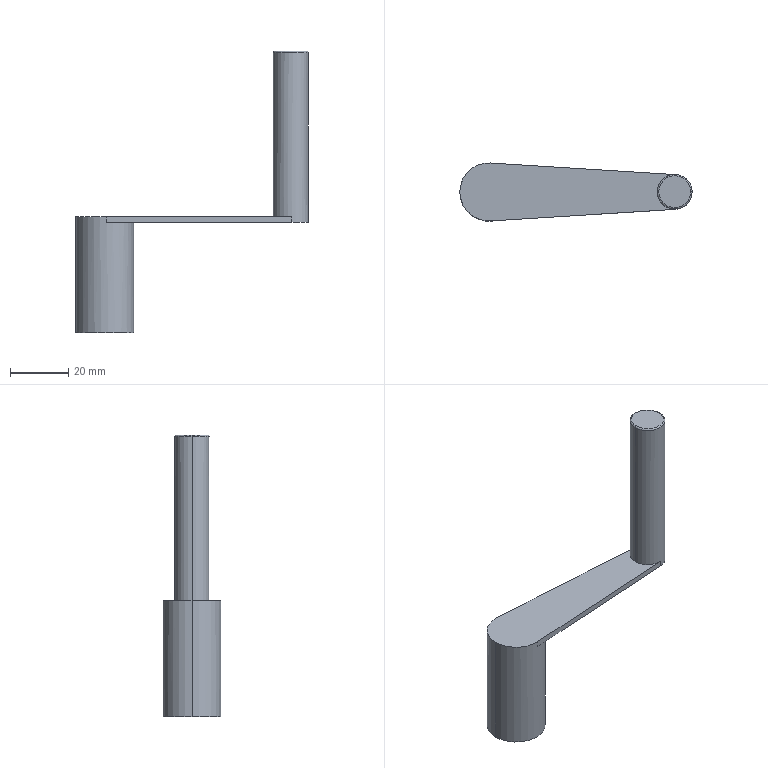Part | STEP file | Z-type Silver Iron Handle | 1 solid | 21 faces | box 80 x 20 x 97 mm | volume 17986 mm3 | plane 11 | cylinder 8 | torus 2 | commonest cylinder face diameters 1 x4 12 x2 20 x2
STEP:
#1=CARTESIAN_POINT('',(0.,0.,0.));
#2=DIRECTION('',(0.,0.,1.));
#3=DIRECTION('',(1.,0.,0.));
#4=AXIS2_PLACEMENT_3D('',#1,#2,#3);
#5=CARTESIAN_POINT('',(58.,0.,96.5));
#6=VERTEX_POINT('',#5);
#7=CARTESIAN_POINT('',(70.,0.,96.5));
#8=VERTEX_POINT('',#7);
#9=CARTESIAN_POINT('',(64.,0.,96.5));
#10=DIRECTION('',(0.,0.,-1.));
#11=DIRECTION('',(1.,0.,0.));
#12=AXIS2_PLACEMENT_3D('',#9,#10,#11);
#13=CIRCLE('',#12,6.);
#14=CARTESIAN_POINT('',(64.,0.,96.5));
#15=DIRECTION('',(0.,0.,1.));
#16=DIRECTION('',(1.,0.,0.));
#17=AXIS2_PLACEMENT_3D('',#14,#15,#16);
#18=TOROIDAL_SURFACE('',#17,5.5,0.5);
#19=CARTESIAN_POINT('',(6.283,0.));
#20=DIRECTION('',(-1.,0.));
#21=VECTOR('',#20,1.);
#22=LINE('',#19,#21);
#23=(GEOMETRIC_REPRESENTATION_CONTEXT(2)PARAMETRIC_REPRESENTATION_CONTEXT()REPRESENTATION_CONTEXT('',''));
#24=DEFINITIONAL_REPRESENTATION('',(#22),#23);
#25=PCURVE('',#18,#24);
#26=CARTESIAN_POINT('',(64.,0.,40.));
#27=DIRECTION('',(0.,0.,-1.));
#28=DIRECTION('',(-1.,0.,0.));
#29=AXIS2_PLACEMENT_3D('',#26,#27,#28);
#30=CYLINDRICAL_SURFACE('',#29,6.);
#31=CARTESIAN_POINT('',(-3.142,-56.5));
#32=DIRECTION('',(1.,0.));
#33=VECTOR('',#32,1.);
#34=LINE('',#31,#33);
#35=(GEOMETRIC_REPRESENTATION_CONTEXT(2)PARAMETRIC_REPRESENTATION_CONTEXT()REPRESENTATION_CONTEXT('',''));
#36=DEFINITIONAL_REPRESENTATION('',(#34),#35);
#37=PCURVE('',#30,#36);
#38=SURFACE_CURVE('',#13,(#25,#37),.PCURVE_S1.);
#39=EDGE_CURVE('',#6,#8,#38,.T.);
#40=ORIENTED_EDGE('',*,*,#39,.F.);
#41=CARTESIAN_POINT('',(58.5,0.,97.));
#42=VERTEX_POINT('',#41);
#43=CARTESIAN_POINT('',(58.5,0.,96.5));
#44=DIRECTION('',(0.,1.,0.));
#45=DIRECTION('',(-1.,0.,0.));
#46=AXIS2_PLACEMENT_3D('',#43,#44,#45);
#47=CIRCLE('',#46,0.5);
#48=CARTESIAN_POINT('',(3.142,0.));
#49=DIRECTION('',(0.,1.));
#50=VECTOR('',#49,1.);
#51=LINE('',#48,#50);
#52=(GEOMETRIC_REPRESENTATION_CONTEXT(2)PARAMETRIC_REPRESENTATION_CONTEXT()REPRESENTATION_CONTEXT('',''));
#53=DEFINITIONAL_REPRESENTATION('',(#51),#52);
#54=PCURVE('',#18,#53);
#55=CARTESIAN_POINT('',(64.,0.,96.5));
#56=DIRECTION('',(0.,0.,1.));
#57=DIRECTION('',(1.,0.,0.));
#58=AXIS2_PLACEMENT_3D('',#55,#56,#57);
#59=TOROIDAL_SURFACE('',#58,5.5,0.5);
#60=CARTESIAN_POINT('',(3.142,0.));
#61=DIRECTION('',(0.,1.));
#62=VECTOR('',#61,1.);
#63=LINE('',#60,#62);
#64=(GEOMETRIC_REPRESENTATION_CONTEXT(2)PARAMETRIC_REPRESENTATION_CONTEXT()REPRESENTATION_CONTEXT('',''));
#65=DEFINITIONAL_REPRESENTATION('',(#63),#64);
#66=PCURVE('',#59,#65);
#67=SURFACE_CURVE('',#47,(#54,#66),.PCURVE_S1.);
#68=EDGE_CURVE('',#6,#42,#67,.T.);
#69=ORIENTED_EDGE('',*,*,#68,.T.);
#70=CARTESIAN_POINT('',(69.5,0.,97.));
#71=VERTEX_POINT('',#70);
#72=CARTESIAN_POINT('',(64.,0.,97.));
#73=DIRECTION('',(0.,0.,1.));
#74=DIRECTION('',(1.,0.,0.));
#75=AXIS2_PLACEMENT_3D('',#72,#73,#74);
#76=CIRCLE('',#75,5.5);
#77=CARTESIAN_POINT('',(0.,1.571));
#78=DIRECTION('',(1.,0.));
#79=VECTOR('',#78,1.);
#80=LINE('',#77,#79);
#81=(GEOMETRIC_REPRESENTATION_CONTEXT(2)PARAMETRIC_REPRESENTATION_CONTEXT()REPRESENTATION_CONTEXT('',''));
#82=DEFINITIONAL_REPRESENTATION('',(#80),#81);
#83=PCURVE('',#18,#82);
#84=CARTESIAN_POINT('',(64.,0.,97.));
#85=DIRECTION('',(0.,0.,1.));
#86=DIRECTION('',(1.,0.,0.));
#87=AXIS2_PLACEMENT_3D('',#84,#85,#86);
#88=PLANE('',#87);
#89=CARTESIAN_POINT('',(0.,0.));
#90=DIRECTION('',(1.,0.));
#91=AXIS2_PLACEMENT_2D('',#89,#90);
#92=CIRCLE('',#91,5.5);
#93=(GEOMETRIC_REPRESENTATION_CONTEXT(2)PARAMETRIC_REPRESENTATION_CONTEXT()REPRESENTATION_CONTEXT('',''));
#94=DEFINITIONAL_REPRESENTATION('',(#92),#93);
#95=PCURVE('',#88,#94);
#96=SURFACE_CURVE('',#76,(#83,#95),.PCURVE_S1.);
#97=EDGE_CURVE('',#71,#42,#96,.T.);
#98=ORIENTED_EDGE('',*,*,#97,.F.);
#99=CARTESIAN_POINT('',(69.5,0.,96.5));
#100=DIRECTION('',(0.,-1.,0.));
#101=DIRECTION('',(0.,0.,-1.));
#102=AXIS2_PLACEMENT_3D('',#99,#100,#101);
#103=CIRCLE('',#102,0.5);
#104=CARTESIAN_POINT('',(0.,-1.571));
#105=DIRECTION('',(0.,1.));
#106=VECTOR('',#105,1.);
#107=LINE('',#104,#106);
#108=(GEOMETRIC_REPRESENTATION_CONTEXT(2)PARAMETRIC_REPRESENTATION_CONTEXT()REPRESENTATION_CONTEXT('',''));
#109=DEFINITIONAL_REPRESENTATION('',(#107),#108);
#110=PCURVE('',#18,#109);
#111=CARTESIAN_POINT('',(6.283,-1.571));
#112=DIRECTION('',(0.,1.));
#113=VECTOR('',#112,1.);
#114=LINE('',#111,#113);
#115=(GEOMETRIC_REPRESENTATION_CONTEXT(2)PARAMETRIC_REPRESENTATION_CONTEXT()REPRESENTATION_CONTEXT('',''));
#116=DEFINITIONAL_REPRESENTATION('',(#114),#115);
#117=PCURVE('',#59,#116);
#118=SURFACE_CURVE('',#103,(#110,#117),.PCURVE_S1.);
#119=EDGE_CURVE('',#8,#71,#118,.T.);
#120=ORIENTED_EDGE('',*,*,#119,.F.);
#121=EDGE_LOOP('',(#40,#69,#98,#120));
#122=FACE_BOUND('',#121,.T.);
#123=ADVANCED_FACE('',(#122),#18,.T.);
#124=ORIENTED_EDGE('',*,*,#39,.T.);
#125=CARTESIAN_POINT('',(70.,0.,38.));
#126=VERTEX_POINT('',#125);
#127=CARTESIAN_POINT('',(70.,0.,40.));
#128=DIRECTION('',(0.,0.,-1.));
#129=VECTOR('',#128,1.);
#130=LINE('',#127,#129);
#131=CARTESIAN_POINT('',(3.142,0.));
#132=DIRECTION('',(0.,1.));
#133=VECTOR('',#132,1.);
#134=LINE('',#131,#133);
#135=(GEOMETRIC_REPRESENTATION_CONTEXT(2)PARAMETRIC_REPRESENTATION_CONTEXT()REPRESENTATION_CONTEXT('',''));
#136=DEFINITIONAL_REPRESENTATION('',(#134),#135);
#137=PCURVE('',#30,#136);
#138=CARTESIAN_POINT('',(64.,0.,40.));
#139=DIRECTION('',(0.,0.,-1.));
#140=DIRECTION('',(-1.,0.,0.));
#141=AXIS2_PLACEMENT_3D('',#138,#139,#140);
#142=CYLINDRICAL_SURFACE('',#141,6.);
#143=CARTESIAN_POINT('',(3.142,0.));
#144=DIRECTION('',(0.,1.));
#145=VECTOR('',#144,1.);
#146=LINE('',#143,#145);
#147=(GEOMETRIC_REPRESENTATION_CONTEXT(2)PARAMETRIC_REPRESENTATION_CONTEXT()REPRESENTATION_CONTEXT('',''));
#148=DEFINITIONAL_REPRESENTATION('',(#146),#147);
#149=PCURVE('',#142,#148);
#150=SURFACE_CURVE('',#130,(#137,#149),.PCURVE_S1.);
#151=EDGE_CURVE('',#8,#126,#150,.T.);
#152=ORIENTED_EDGE('',*,*,#151,.T.);
#153=CARTESIAN_POINT('',(64.375,5.988,38.));
#154=VERTEX_POINT('',#153);
#155=CARTESIAN_POINT('',(64.,0.,38.));
#156=DIRECTION('',(0.,0.,1.));
#157=DIRECTION('',(1.,0.,0.));
#158=AXIS2_PLACEMENT_3D('',#155,#156,#157);
#159=CIRCLE('',#158,6.);
#160=CARTESIAN_POINT('',(3.142,2.));
#161=DIRECTION('',(-1.,0.));
#162=VECTOR('',#161,1.);
#163=LINE('',#160,#162);
#164=(GEOMETRIC_REPRESENTATION_CONTEXT(2)PARAMETRIC_REPRESENTATION_CONTEXT()REPRESENTATION_CONTEXT('',''));
#165=DEFINITIONAL_REPRESENTATION('',(#163),#164);
#166=PCURVE('',#30,#165);
#167=CARTESIAN_POINT('',(64.,0.,38.));
#168=DIRECTION('',(0.,0.,1.));
#169=DIRECTION('',(1.,0.,0.));
#170=AXIS2_PLACEMENT_3D('',#167,#168,#169);
#171=PLANE('',#170);
#172=CARTESIAN_POINT('',(0.,0.));
#173=DIRECTION('',(1.,0.));
#174=AXIS2_PLACEMENT_2D('',#172,#173);
#175=CIRCLE('',#174,6.);
#176=(GEOMETRIC_REPRESENTATION_CONTEXT(2)PARAMETRIC_REPRESENTATION_CONTEXT()REPRESENTATION_CONTEXT('',''));
#177=DEFINITIONAL_REPRESENTATION('',(#175),#176);
#178=PCURVE('',#171,#177);
#179=SURFACE_CURVE('',#159,(#166,#178),.PCURVE_S1.);
#180=EDGE_CURVE('',#126,#154,#179,.T.);
#181=ORIENTED_EDGE('',*,*,#180,.T.);
#182=CARTESIAN_POINT('',(64.375,5.988,40.));
#183=VERTEX_POINT('',#182);
#184=CARTESIAN_POINT('',(64.375,5.988,40.));
#185=DIRECTION('',(0.,0.,-1.));
#186=VECTOR('',#185,1.);
#187=LINE('',#184,#186);
#188=CARTESIAN_POINT('',(1.633,0.));
#189=DIRECTION('',(0.,1.));
#190=VECTOR('',#189,1.);
#191=LINE('',#188,#190);
#192=(GEOMETRIC_REPRESENTATION_CONTEXT(2)PARAMETRIC_REPRESENTATION_CONTEXT()REPRESENTATION_CONTEXT('',''));
#193=DEFINITIONAL_REPRESENTATION('',(#191),#192);
#194=PCURVE('',#30,#193);
#195=CARTESIAN_POINT('',(0.625,9.98,40.));
#196=DIRECTION('',(-0.0625,-0.998,0.));
#197=DIRECTION('',(0.998,-0.0625,0.));
#198=AXIS2_PLACEMENT_3D('',#195,#196,#197);
#199=PLANE('',#198);
#200=CARTESIAN_POINT('',(63.875,0.));
#201=DIRECTION('',(0.,-1.));
#202=VECTOR('',#201,1.);
#203=LINE('',#200,#202);
#204=(GEOMETRIC_REPRESENTATION_CONTEXT(2)PARAMETRIC_REPRESENTATION_CONTEXT()REPRESENTATION_CONTEXT('',''));
#205=DEFINITIONAL_REPRESENTATION('',(#203),#204);
#206=PCURVE('',#199,#205);
#207=SURFACE_CURVE('',#187,(#194,#206),.PCURVE_S1.);
#208=EDGE_CURVE('',#183,#154,#207,.T.);
#209=ORIENTED_EDGE('',*,*,#208,.F.);
#210=CARTESIAN_POINT('',(58.,0.,40.));
#211=VERTEX_POINT('',#210);
#212=CARTESIAN_POINT('',(64.,0.,40.));
#213=DIRECTION('',(0.,0.,1.));
#214=DIRECTION('',(1.,0.,0.));
#215=AXIS2_PLACEMENT_3D('',#212,#213,#214);
#216=CIRCLE('',#215,6.);
#217=CARTESIAN_POINT('',(3.142,0.));
#218=DIRECTION('',(-1.,0.));
#219=VECTOR('',#218,1.);
#220=LINE('',#217,#219);
#221=(GEOMETRIC_REPRESENTATION_CONTEXT(2)PARAMETRIC_REPRESENTATION_CONTEXT()REPRESENTATION_CONTEXT('',''));
#222=DEFINITIONAL_REPRESENTATION('',(#220),#221);
#223=PCURVE('',#30,#222);
#224=CARTESIAN_POINT('',(64.,0.,40.));
#225=DIRECTION('',(0.,0.,1.));
#226=DIRECTION('',(1.,0.,0.));
#227=AXIS2_PLACEMENT_3D('',#224,#225,#226);
#228=PLANE('',#227);
#229=CARTESIAN_POINT('',(0.,0.));
#230=DIRECTION('',(1.,0.));
#231=AXIS2_PLACEMENT_2D('',#229,#230);
#232=CIRCLE('',#231,6.);
#233=(GEOMETRIC_REPRESENTATION_CONTEXT(2)PARAMETRIC_REPRESENTATION_CONTEXT()REPRESENTATION_CONTEXT('',''));
#234=DEFINITIONAL_REPRESENTATION('',(#232),#233);
#235=PCURVE('',#228,#234);
#236=SURFACE_CURVE('',#216,(#223,#235),.PCURVE_S1.);
#237=EDGE_CURVE('',#183,#211,#236,.T.);
#238=ORIENTED_EDGE('',*,*,#237,.T.);
#239=CARTESIAN_POINT('',(58.,0.,40.));
#240=DIRECTION('',(0.,0.,-1.));
#241=VECTOR('',#240,1.);
#242=LINE('',#239,#241);
#243=CARTESIAN_POINT('',(0.,0.));
#244=DIRECTION('',(0.,1.));
#245=VECTOR('',#244,1.);
#246=LINE('',#243,#245);
#247=(GEOMETRIC_REPRESENTATION_CONTEXT(2)PARAMETRIC_REPRESENTATION_CONTEXT()REPRESENTATION_CONTEXT('',''));
#248=DEFINITIONAL_REPRESENTATION('',(#246),#247);
#249=PCURVE('',#30,#248);
#250=CARTESIAN_POINT('',(6.283,0.));
#251=DIRECTION('',(0.,1.));
#252=VECTOR('',#251,1.);
#253=LINE('',#250,#252);
#254=(GEOMETRIC_REPRESENTATION_CONTEXT(2)PARAMETRIC_REPRESENTATION_CONTEXT()REPRESENTATION_CONTEXT('',''));
#255=DEFINITIONAL_REPRESENTATION('',(#253),#254);
#256=PCURVE('',#142,#255);
#257=SURFACE_CURVE('',#242,(#249,#256),.PCURVE_S1.);
#258=EDGE_CURVE('',#6,#211,#257,.T.);
#259=ORIENTED_EDGE('',*,*,#258,.F.);
#260=EDGE_LOOP('',(#124,#152,#181,#209,#238,#259));
#261=FACE_BOUND('',#260,.T.);
#262=ADVANCED_FACE('',(#261),#30,.T.);
#263=CARTESIAN_POINT('',(10.,0.,38.));
#264=VERTEX_POINT('',#263);
#265=CARTESIAN_POINT('',(0.625,9.98,38.));
#266=VERTEX_POINT('',#265);
#267=CARTESIAN_POINT('',(0.,0.,38.));
#268=DIRECTION('',(0.,0.,1.));
#269=DIRECTION('',(1.,0.,0.));
#270=AXIS2_PLACEMENT_3D('',#267,#268,#269);
#271=CIRCLE('',#270,10.);
#272=CARTESIAN_POINT('',(0.,0.,38.));
#273=DIRECTION('',(0.,0.,-1.));
#274=DIRECTION('',(-1.,0.,0.));
#275=AXIS2_PLACEMENT_3D('',#272,#273,#274);
#276=CYLINDRICAL_SURFACE('',#275,10.);
#277=CARTESIAN_POINT('',(3.142,0.));
#278=DIRECTION('',(-1.,0.));
#279=VECTOR('',#278,1.);
#280=LINE('',#277,#279);
#281=(GEOMETRIC_REPRESENTATION_CONTEXT(2)PARAMETRIC_REPRESENTATION_CONTEXT()REPRESENTATION_CONTEXT('',''));
#282=DEFINITIONAL_REPRESENTATION('',(#280),#281);
#283=PCURVE('',#276,#282);
#284=CARTESIAN_POINT('',(-64.,0.));
#285=DIRECTION('',(1.,0.));
#286=AXIS2_PLACEMENT_2D('',#284,#285);
#287=CIRCLE('',#286,10.);
#288=(GEOMETRIC_REPRESENTATION_CONTEXT(2)PARAMETRIC_REPRESENTATION_CONTEXT()REPRESENTATION_CONTEXT('',''));
#289=DEFINITIONAL_REPRESENTATION('',(#287),#288);
#290=PCURVE('',#171,#289);
#291=SURFACE_CURVE('',#271,(#283,#290),.PCURVE_S1.);
#292=EDGE_CURVE('',#264,#266,#291,.T.);
#293=ORIENTED_EDGE('',*,*,#292,.F.);
#294=CARTESIAN_POINT('',(10.,0.,0.));
#295=VERTEX_POINT('',#294);
#296=CARTESIAN_POINT('',(10.,0.,38.));
#297=DIRECTION('',(0.,0.,-1.));
#298=VECTOR('',#297,1.);
#299=LINE('',#296,#298);
#300=CARTESIAN_POINT('',(3.142,0.));
#301=DIRECTION('',(0.,1.));
#302=VECTOR('',#301,1.);
#303=LINE('',#300,#302);
#304=(GEOMETRIC_REPRESENTATION_CONTEXT(2)PARAMETRIC_REPRESENTATION_CONTEXT()REPRESENTATION_CONTEXT('',''));
#305=DEFINITIONAL_REPRESENTATION('',(#303),#304);
#306=PCURVE('',#276,#305);
#307=CARTESIAN_POINT('',(0.,0.,38.));
#308=DIRECTION('',(0.,0.,-1.));
#309=DIRECTION('',(-1.,0.,0.));
#310=AXIS2_PLACEMENT_3D('',#307,#308,#309);
#311=CYLINDRICAL_SURFACE('',#310,10.);
#312=CARTESIAN_POINT('',(3.142,0.));
#313=DIRECTION('',(0.,1.));
#314=VECTOR('',#313,1.);
#315=LINE('',#312,#314);
#316=(GEOMETRIC_REPRESENTATION_CONTEXT(2)PARAMETRIC_REPRESENTATION_CONTEXT()REPRESENTATION_CONTEXT('',''));
#317=DEFINITIONAL_REPRESENTATION('',(#315),#316);
#318=PCURVE('',#311,#317);
#319=SURFACE_CURVE('',#299,(#306,#318),.PCURVE_S1.);
#320=EDGE_CURVE('',#264,#295,#319,.T.);
#321=ORIENTED_EDGE('',*,*,#320,.T.);
#322=CARTESIAN_POINT('',(-10.,0.,0.));
#323=VERTEX_POINT('',#322);
#324=CARTESIAN_POINT('',(0.,0.,0.));
#325=DIRECTION('',(0.,0.,1.));
#326=DIRECTION('',(1.,0.,0.));
#327=AXIS2_PLACEMENT_3D('',#324,#325,#326);
#328=CIRCLE('',#327,10.);
#329=CARTESIAN_POINT('',(3.142,38.));
#330=DIRECTION('',(-1.,0.));
#331=VECTOR('',#330,1.);
#332=LINE('',#329,#331);
#333=(GEOMETRIC_REPRESENTATION_CONTEXT(2)PARAMETRIC_REPRESENTATION_CONTEXT()REPRESENTATION_CONTEXT('',''));
#334=DEFINITIONAL_REPRESENTATION('',(#332),#333);
#335=PCURVE('',#276,#334);
#336=CARTESIAN_POINT('',(0.,0.,0.));
#337=DIRECTION('',(0.,0.,1.));
#338=DIRECTION('',(1.,0.,0.));
#339=AXIS2_PLACEMENT_3D('',#336,#337,#338);
#340=PLANE('',#339);
#341=CARTESIAN_POINT('',(0.,0.));
#342=DIRECTION('',(1.,0.));
#343=AXIS2_PLACEMENT_2D('',#341,#342);
#344=CIRCLE('',#343,10.);
#345=(GEOMETRIC_REPRESENTATION_CONTEXT(2)PARAMETRIC_REPRESENTATION_CONTEXT()REPRESENTATION_CONTEXT('',''));
#346=DEFINITIONAL_REPRESENTATION('',(#344),#345);
#347=PCURVE('',#340,#346);
#348=SURFACE_CURVE('',#328,(#335,#347),.PCURVE_S1.);
#349=EDGE_CURVE('',#295,#323,#348,.T.);
#350=ORIENTED_EDGE('',*,*,#349,.T.);
#351=CARTESIAN_POINT('',(-10.,0.,40.));
#352=VERTEX_POINT('',#351);
#353=CARTESIAN_POINT('',(-10.,0.,38.));
#354=DIRECTION('',(0.,0.,-1.));
#355=VECTOR('',#354,1.);
#356=LINE('',#353,#355);
#357=CARTESIAN_POINT('',(0.,0.));
#358=DIRECTION('',(0.,1.));
#359=VECTOR('',#358,1.);
#360=LINE('',#357,#359);
#361=(GEOMETRIC_REPRESENTATION_CONTEXT(2)PARAMETRIC_REPRESENTATION_CONTEXT()REPRESENTATION_CONTEXT('',''));
#362=DEFINITIONAL_REPRESENTATION('',(#360),#361);
#363=PCURVE('',#276,#362);
#364=CARTESIAN_POINT('',(6.283,0.));
#365=DIRECTION('',(0.,1.));
#366=VECTOR('',#365,1.);
#367=LINE('',#364,#366);
#368=(GEOMETRIC_REPRESENTATION_CONTEXT(2)PARAMETRIC_REPRESENTATION_CONTEXT()REPRESENTATION_CONTEXT('',''));
#369=DEFINITIONAL_REPRESENTATION('',(#367),#368);
#370=PCURVE('',#311,#369);
#371=SURFACE_CURVE('',#356,(#363,#370),.PCURVE_S1.);
#372=EDGE_CURVE('',#352,#323,#371,.T.);
#373=ORIENTED_EDGE('',*,*,#372,.F.);
#374=CARTESIAN_POINT('',(0.625,9.98,40.));
#375=VERTEX_POINT('',#374);
#376=CARTESIAN_POINT('',(0.,0.,40.));
#377=DIRECTION('',(0.,0.,1.));
#378=DIRECTION('',(1.,0.,0.));
#379=AXIS2_PLACEMENT_3D('',#376,#377,#378);
#380=CIRCLE('',#379,10.);
#381=CARTESIAN_POINT('',(3.142,-2.));
#382=DIRECTION('',(-1.,0.));
#383=VECTOR('',#382,1.);
#384=LINE('',#381,#383);
#385=(GEOMETRIC_REPRESENTATION_CONTEXT(2)PARAMETRIC_REPRESENTATION_CONTEXT()REPRESENTATION_CONTEXT('',''));
#386=DEFINITIONAL_REPRESENTATION('',(#384),#385);
#387=PCURVE('',#276,#386);
#388=CARTESIAN_POINT('',(-64.,0.));
#389=DIRECTION('',(1.,0.));
#390=AXIS2_PLACEMENT_2D('',#388,#389);
#391=CIRCLE('',#390,10.);
#392=(GEOMETRIC_REPRESENTATION_CONTEXT(2)PARAMETRIC_REPRESENTATION_CONTEXT()REPRESENTATION_CONTEXT('',''));
#393=DEFINITIONAL_REPRESENTATION('',(#391),#392);
#394=PCURVE('',#228,#393);
#395=SURFACE_CURVE('',#380,(#387,#394),.PCURVE_S1.);
#396=EDGE_CURVE('',#375,#352,#395,.T.);
#397=ORIENTED_EDGE('',*,*,#396,.F.);
#398=CARTESIAN_POINT('',(0.625,9.98,40.));
#399=DIRECTION('',(0.,0.,-1.));
#400=VECTOR('',#399,1.);
#401=LINE('',#398,#400);
#402=CARTESIAN_POINT('',(1.633,-2.));
#403=DIRECTION('',(0.,1.));
#404=VECTOR('',#403,1.);
#405=LINE('',#402,#404);
#406=(GEOMETRIC_REPRESENTATION_CONTEXT(2)PARAMETRIC_REPRESENTATION_CONTEXT()REPRESENTATION_CONTEXT('',''));
#407=DEFINITIONAL_REPRESENTATION('',(#405),#406);
#408=PCURVE('',#276,#407);
#409=CARTESIAN_POINT('',(0.,0.));
#410=DIRECTION('',(0.,-1.));
#411=VECTOR('',#410,1.);
#412=LINE('',#409,#411);
#413=(GEOMETRIC_REPRESENTATION_CONTEXT(2)PARAMETRIC_REPRESENTATION_CONTEXT()REPRESENTATION_CONTEXT('',''));
#414=DEFINITIONAL_REPRESENTATION('',(#412),#413);
#415=PCURVE('',#199,#414);
#416=SURFACE_CURVE('',#401,(#408,#415),.PCURVE_S1.);
#417=EDGE_CURVE('',#375,#266,#416,.T.);
#418=ORIENTED_EDGE('',*,*,#417,.T.);
#419=EDGE_LOOP('',(#293,#321,#350,#373,#397,#418));
#420=FACE_BOUND('',#419,.T.);
#421=ADVANCED_FACE('',(#420),#276,.T.);
#422=ORIENTED_EDGE('',*,*,#320,.F.);
#423=CARTESIAN_POINT('',(0.625,-9.98,38.));
#424=VERTEX_POINT('',#423);
#425=CARTESIAN_POINT('',(0.,0.,38.));
#426=DIRECTION('',(0.,0.,1.));
#427=DIRECTION('',(1.,0.,0.));
#428=AXIS2_PLACEMENT_3D('',#425,#426,#427);
#429=CIRCLE('',#428,10.);
#430=CARTESIAN_POINT('',(9.425,0.));
#431=DIRECTION('',(-1.,0.));
#432=VECTOR('',#431,1.);
#433=LINE('',#430,#432);
#434=(GEOMETRIC_REPRESENTATION_CONTEXT(2)PARAMETRIC_REPRESENTATION_CONTEXT()REPRESENTATION_CONTEXT('',''));
#435=DEFINITIONAL_REPRESENTATION('',(#433),#434);
#436=PCURVE('',#311,#435);
#437=CARTESIAN_POINT('',(-64.,0.));
#438=DIRECTION('',(1.,0.));
#439=AXIS2_PLACEMENT_2D('',#437,#438);
#440=CIRCLE('',#439,10.);
#441=(GEOMETRIC_REPRESENTATION_CONTEXT(2)PARAMETRIC_REPRESENTATION_CONTEXT()REPRESENTATION_CONTEXT('',''));
#442=DEFINITIONAL_REPRESENTATION('',(#440),#441);
#443=PCURVE('',#171,#442);
#444=SURFACE_CURVE('',#429,(#436,#443),.PCURVE_S1.);
#445=EDGE_CURVE('',#424,#264,#444,.T.);
#446=ORIENTED_EDGE('',*,*,#445,.F.);
#447=CARTESIAN_POINT('',(0.625,-9.98,40.));
#448=VERTEX_POINT('',#447);
#449=CARTESIAN_POINT('',(0.625,-9.98,40.));
#450=DIRECTION('',(0.,0.,-1.));
#451=VECTOR('',#450,1.);
#452=LINE('',#449,#451);
#453=CARTESIAN_POINT('',(4.65,-2.));
#454=DIRECTION('',(0.,1.));
#455=VECTOR('',#454,1.);
#456=LINE('',#453,#455);
#457=(GEOMETRIC_REPRESENTATION_CONTEXT(2)PARAMETRIC_REPRESENTATION_CONTEXT()REPRESENTATION_CONTEXT('',''));
#458=DEFINITIONAL_REPRESENTATION('',(#456),#457);
#459=PCURVE('',#311,#458);
#460=CARTESIAN_POINT('',(64.375,-5.988,40.));
#461=DIRECTION('',(-0.0625,0.998,0.));
#462=DIRECTION('',(-0.998,-0.0625,0.));
#463=AXIS2_PLACEMENT_3D('',#460,#461,#462);
#464=PLANE('',#463);
#465=CARTESIAN_POINT('',(63.875,0.));
#466=DIRECTION('',(0.,-1.));
#467=VECTOR('',#466,1.);
#468=LINE('',#465,#467);
#469=(GEOMETRIC_REPRESENTATION_CONTEXT(2)PARAMETRIC_REPRESENTATION_CONTEXT()REPRESENTATION_CONTEXT('',''));
#470=DEFINITIONAL_REPRESENTATION('',(#468),#469);
#471=PCURVE('',#464,#470);
#472=SURFACE_CURVE('',#452,(#459,#471),.PCURVE_S1.);
#473=EDGE_CURVE('',#448,#424,#472,.T.);
#474=ORIENTED_EDGE('',*,*,#473,.F.);
#475=CARTESIAN_POINT('',(0.,0.,40.));
#476=DIRECTION('',(0.,0.,1.));
#477=DIRECTION('',(1.,0.,0.));
#478=AXIS2_PLACEMENT_3D('',#475,#476,#477);
#479=CIRCLE('',#478,10.);
#480=CARTESIAN_POINT('',(9.425,-2.));
#481=DIRECTION('',(-1.,0.));
#482=VECTOR('',#481,1.);
#483=LINE('',#480,#482);
#484=(GEOMETRIC_REPRESENTATION_CONTEXT(2)PARAMETRIC_REPRESENTATION_CONTEXT()REPRESENTATION_CONTEXT('',''));
#485=DEFINITIONAL_REPRESENTATION('',(#483),#484);
#486=PCURVE('',#311,#485);
#487=CARTESIAN_POINT('',(-64.,0.));
#488=DIRECTION('',(1.,0.));
#489=AXIS2_PLACEMENT_2D('',#487,#488);
#490=CIRCLE('',#489,10.);
#491=(GEOMETRIC_REPRESENTATION_CONTEXT(2)PARAMETRIC_REPRESENTATION_CONTEXT()REPRESENTATION_CONTEXT('',''));
#492=DEFINITIONAL_REPRESENTATION('',(#490),#491);
#493=PCURVE('',#228,#492);
#494=SURFACE_CURVE('',#479,(#486,#493),.PCURVE_S1.);
#495=EDGE_CURVE('',#352,#448,#494,.T.);
#496=ORIENTED_EDGE('',*,*,#495,.F.);
#497=ORIENTED_EDGE('',*,*,#372,.T.);
#498=CARTESIAN_POINT('',(0.,0.,0.));
#499=DIRECTION('',(0.,0.,1.));
#500=DIRECTION('',(1.,0.,0.));
#501=AXIS2_PLACEMENT_3D('',#498,#499,#500);
#502=CIRCLE('',#501,10.);
#503=CARTESIAN_POINT('',(9.425,38.));
#504=DIRECTION('',(-1.,0.));
#505=VECTOR('',#504,1.);
#506=LINE('',#503,#505);
#507=(GEOMETRIC_REPRESENTATION_CONTEXT(2)PARAMETRIC_REPRESENTATION_CONTEXT()REPRESENTATION_CONTEXT('',''));
#508=DEFINITIONAL_REPRESENTATION('',(#506),#507);
#509=PCURVE('',#311,#508);
#510=CARTESIAN_POINT('',(0.,0.));
#511=DIRECTION('',(1.,0.));
#512=AXIS2_PLACEMENT_2D('',#510,#511);
#513=CIRCLE('',#512,10.);
#514=(GEOMETRIC_REPRESENTATION_CONTEXT(2)PARAMETRIC_REPRESENTATION_CONTEXT()REPRESENTATION_CONTEXT('',''));
#515=DEFINITIONAL_REPRESENTATION('',(#513),#514);
#516=PCURVE('',#340,#515);
#517=SURFACE_CURVE('',#502,(#509,#516),.PCURVE_S1.);
#518=EDGE_CURVE('',#323,#295,#517,.T.);
#519=ORIENTED_EDGE('',*,*,#518,.T.);
#520=EDGE_LOOP('',(#422,#446,#474,#496,#497,#519));
#521=FACE_BOUND('',#520,.T.);
#522=ADVANCED_FACE('',(#521),#311,.T.);
#523=CARTESIAN_POINT('',(-5.5,6.,0.));
#524=VERTEX_POINT('',#523);
#525=CARTESIAN_POINT('',(5.5,6.,0.));
#526=VERTEX_POINT('',#525);
#527=CARTESIAN_POINT('',(6.,6.,0.));
#528=DIRECTION('',(1.,0.,0.));
#529=VECTOR('',#528,1.);
#530=LINE('',#527,#529);
#531=CARTESIAN_POINT('',(6.,6.));
#532=DIRECTION('',(1.,0.));
#533=VECTOR('',#532,1.);
#534=LINE('',#531,#533);
#535=(GEOMETRIC_REPRESENTATION_CONTEXT(2)PARAMETRIC_REPRESENTATION_CONTEXT()REPRESENTATION_CONTEXT('',''));
#536=DEFINITIONAL_REPRESENTATION('',(#534),#535);
#537=PCURVE('',#340,#536);
#538=CARTESIAN_POINT('',(6.,6.,20.));
#539=DIRECTION('',(0.,1.,0.));
#540=DIRECTION('',(0.,0.,1.));
#541=AXIS2_PLACEMENT_3D('',#538,#539,#540);
#542=PLANE('',#541);
#543=CARTESIAN_POINT('',(-20.,0.));
#544=DIRECTION('',(0.,1.));
#545=VECTOR('',#544,1.);
#546=LINE('',#543,#545);
#547=(GEOMETRIC_REPRESENTATION_CONTEXT(2)PARAMETRIC_REPRESENTATION_CONTEXT()REPRESENTATION_CONTEXT('',''));
#548=DEFINITIONAL_REPRESENTATION('',(#546),#547);
#549=PCURVE('',#542,#548);
#550=SURFACE_CURVE('',#530,(#537,#549),.PCURVE_S1.);
#551=EDGE_CURVE('',#524,#526,#550,.T.);
#552=ORIENTED_EDGE('',*,*,#551,.F.);
#553=CARTESIAN_POINT('',(-6.,5.5,0.));
#554=VERTEX_POINT('',#553);
#555=CARTESIAN_POINT('',(-5.5,5.5,0.));
#556=DIRECTION('',(0.,0.,1.));
#557=DIRECTION('',(1.,0.,0.));
#558=AXIS2_PLACEMENT_3D('',#555,#556,#557);
#559=CIRCLE('',#558,0.5);
#560=CARTESIAN_POINT('',(-5.5,5.5));
#561=DIRECTION('',(1.,0.));
#562=AXIS2_PLACEMENT_2D('',#560,#561);
#563=CIRCLE('',#562,0.5);
#564=(GEOMETRIC_REPRESENTATION_CONTEXT(2)PARAMETRIC_REPRESENTATION_CONTEXT()REPRESENTATION_CONTEXT('',''));
#565=DEFINITIONAL_REPRESENTATION('',(#563),#564);
#566=PCURVE('',#340,#565);
#567=CARTESIAN_POINT('',(-5.5,5.5,20.));
#568=DIRECTION('',(0.,0.,1.));
#569=DIRECTION('',(1.,0.,0.));
#570=AXIS2_PLACEMENT_3D('',#567,#568,#569);
#571=CYLINDRICAL_SURFACE('',#570,0.5);
#572=CARTESIAN_POINT('',(0.,-20.));
#573=DIRECTION('',(1.,0.));
#574=VECTOR('',#573,1.);
#575=LINE('',#572,#574);
#576=(GEOMETRIC_REPRESENTATION_CONTEXT(2)PARAMETRIC_REPRESENTATION_CONTEXT()REPRESENTATION_CONTEXT('',''));
#577=DEFINITIONAL_REPRESENTATION('',(#575),#576);
#578=PCURVE('',#571,#577);
#579=SURFACE_CURVE('',#559,(#566,#578),.PCURVE_S1.);
#580=EDGE_CURVE('',#524,#554,#579,.T.);
#581=ORIENTED_EDGE('',*,*,#580,.T.);
#582=CARTESIAN_POINT('',(-6.,-5.5,0.));
#583=VERTEX_POINT('',#582);
#584=CARTESIAN_POINT('',(-6.,6.,0.));
#585=DIRECTION('',(0.,1.,0.));
#586=VECTOR('',#585,1.);
#587=LINE('',#584,#586);
#588=CARTESIAN_POINT('',(-6.,6.));
#589=DIRECTION('',(0.,1.));
#590=VECTOR('',#589,1.);
#591=LINE('',#588,#590);
#592=(GEOMETRIC_REPRESENTATION_CONTEXT(2)PARAMETRIC_REPRESENTATION_CONTEXT()REPRESENTATION_CONTEXT('',''));
#593=DEFINITIONAL_REPRESENTATION('',(#591),#592);
#594=PCURVE('',#340,#593);
#595=CARTESIAN_POINT('',(-6.,6.,20.));
#596=DIRECTION('',(-1.,0.,0.));
#597=DIRECTION('',(0.,-1.,0.));
#598=AXIS2_PLACEMENT_3D('',#595,#596,#597);
#599=PLANE('',#598);
#600=CARTESIAN_POINT('',(0.,-20.));
#601=DIRECTION('',(-1.,0.));
#602=VECTOR('',#601,1.);
#603=LINE('',#600,#602);
#604=(GEOMETRIC_REPRESENTATION_CONTEXT(2)PARAMETRIC_REPRESENTATION_CONTEXT()REPRESENTATION_CONTEXT('',''));
#605=DEFINITIONAL_REPRESENTATION('',(#603),#604);
#606=PCURVE('',#599,#605);
#607=SURFACE_CURVE('',#587,(#594,#606),.PCURVE_S1.);
#608=EDGE_CURVE('',#583,#554,#607,.T.);
#609=ORIENTED_EDGE('',*,*,#608,.F.);
#610=CARTESIAN_POINT('',(-5.5,-6.,0.));
#611=VERTEX_POINT('',#610);
#612=CARTESIAN_POINT('',(-5.5,-5.5,0.));
#613=DIRECTION('',(0.,0.,1.));
#614=DIRECTION('',(1.,0.,0.));
#615=AXIS2_PLACEMENT_3D('',#612,#613,#614);
#616=CIRCLE('',#615,0.5);
#617=CARTESIAN_POINT('',(-5.5,-5.5));
#618=DIRECTION('',(1.,0.));
#619=AXIS2_PLACEMENT_2D('',#617,#618);
#620=CIRCLE('',#619,0.5);
#621=(GEOMETRIC_REPRESENTATION_CONTEXT(2)PARAMETRIC_REPRESENTATION_CONTEXT()REPRESENTATION_CONTEXT('',''));
#622=DEFINITIONAL_REPRESENTATION('',(#620),#621);
#623=PCURVE('',#340,#622);
#624=CARTESIAN_POINT('',(-5.5,-5.5,20.));
#625=DIRECTION('',(0.,0.,1.));
#626=DIRECTION('',(1.,0.,0.));
#627=AXIS2_PLACEMENT_3D('',#624,#625,#626);
#628=CYLINDRICAL_SURFACE('',#627,0.5);
#629=CARTESIAN_POINT('',(0.,-20.));
#630=DIRECTION('',(1.,0.));
#631=VECTOR('',#630,1.);
#632=LINE('',#629,#631);
#633=(GEOMETRIC_REPRESENTATION_CONTEXT(2)PARAMETRIC_REPRESENTATION_CONTEXT()REPRESENTATION_CONTEXT('',''));
#634=DEFINITIONAL_REPRESENTATION('',(#632),#633);
#635=PCURVE('',#628,#634);
#636=SURFACE_CURVE('',#616,(#623,#635),.PCURVE_S1.);
#637=EDGE_CURVE('',#583,#611,#636,.T.);
#638=ORIENTED_EDGE('',*,*,#637,.T.);
#639=CARTESIAN_POINT('',(5.5,-6.,0.));
#640=VERTEX_POINT('',#639);
#641=CARTESIAN_POINT('',(6.,-6.,0.));
#642=DIRECTION('',(-1.,0.,0.));
#643=VECTOR('',#642,1.);
#644=LINE('',#641,#643);
#645=CARTESIAN_POINT('',(6.,-6.));
#646=DIRECTION('',(-1.,0.));
#647=VECTOR('',#646,1.);
#648=LINE('',#645,#647);
#649=(GEOMETRIC_REPRESENTATION_CONTEXT(2)PARAMETRIC_REPRESENTATION_CONTEXT()REPRESENTATION_CONTEXT('',''));
#650=DEFINITIONAL_REPRESENTATION('',(#648),#649);
#651=PCURVE('',#340,#650);
#652=CARTESIAN_POINT('',(6.,-6.,20.));
#653=DIRECTION('',(0.,-1.,0.));
#654=DIRECTION('',(0.,0.,-1.));
#655=AXIS2_PLACEMENT_3D('',#652,#653,#654);
#656=PLANE('',#655);
#657=CARTESIAN_POINT('',(20.,0.));
#658=DIRECTION('',(0.,-1.));
#659=VECTOR('',#658,1.);
#660=LINE('',#657,#659);
#661=(GEOMETRIC_REPRESENTATION_CONTEXT(2)PARAMETRIC_REPRESENTATION_CONTEXT()REPRESENTATION_CONTEXT('',''));
#662=DEFINITIONAL_REPRESENTATION('',(#660),#661);
#663=PCURVE('',#656,#662);
#664=SURFACE_CURVE('',#644,(#651,#663),.PCURVE_S1.);
#665=EDGE_CURVE('',#640,#611,#664,.T.);
#666=ORIENTED_EDGE('',*,*,#665,.F.);
#667=CARTESIAN_POINT('',(6.,-5.5,0.));
#668=VERTEX_POINT('',#667);
#669=CARTESIAN_POINT('',(5.5,-5.5,0.));
#670=DIRECTION('',(0.,0.,1.));
#671=DIRECTION('',(1.,0.,0.));
#672=AXIS2_PLACEMENT_3D('',#669,#670,#671);
#673=CIRCLE('',#672,0.5);
#674=CARTESIAN_POINT('',(5.5,-5.5));
#675=DIRECTION('',(1.,0.));
#676=AXIS2_PLACEMENT_2D('',#674,#675);
#677=CIRCLE('',#676,0.5);
#678=(GEOMETRIC_REPRESENTATION_CONTEXT(2)PARAMETRIC_REPRESENTATION_CONTEXT()REPRESENTATION_CONTEXT('',''));
#679=DEFINITIONAL_REPRESENTATION('',(#677),#678);
#680=PCURVE('',#340,#679);
#681=CARTESIAN_POINT('',(5.5,-5.5,20.));
#682=DIRECTION('',(0.,0.,1.));
#683=DIRECTION('',(1.,0.,0.));
#684=AXIS2_PLACEMENT_3D('',#681,#682,#683);
#685=CYLINDRICAL_SURFACE('',#684,0.5);
#686=CARTESIAN_POINT('',(0.,-20.));
#687=DIRECTION('',(1.,0.));
#688=VECTOR('',#687,1.);
#689=LINE('',#686,#688);
#690=(GEOMETRIC_REPRESENTATION_CONTEXT(2)PARAMETRIC_REPRESENTATION_CONTEXT()REPRESENTATION_CONTEXT('',''));
#691=DEFINITIONAL_REPRESENTATION('',(#689),#690);
#692=PCURVE('',#685,#691);
#693=SURFACE_CURVE('',#673,(#680,#692),.PCURVE_S1.);
#694=EDGE_CURVE('',#640,#668,#693,.T.);
#695=ORIENTED_EDGE('',*,*,#694,.T.);
#696=CARTESIAN_POINT('',(6.,5.5,0.));
#697=VERTEX_POINT('',#696);
#698=CARTESIAN_POINT('',(6.,6.,0.));
#699=DIRECTION('',(0.,-1.,0.));
#700=VECTOR('',#699,1.);
#701=LINE('',#698,#700);
#702=CARTESIAN_POINT('',(6.,6.));
#703=DIRECTION('',(0.,-1.));
#704=VECTOR('',#703,1.);
#705=LINE('',#702,#704);
#706=(GEOMETRIC_REPRESENTATION_CONTEXT(2)PARAMETRIC_REPRESENTATION_CONTEXT()REPRESENTATION_CONTEXT('',''));
#707=DEFINITIONAL_REPRESENTATION('',(#705),#706);
#708=PCURVE('',#340,#707);
#709=CARTESIAN_POINT('',(6.,6.,20.));
#710=DIRECTION('',(1.,0.,0.));
#711=DIRECTION('',(0.,1.,0.));
#712=AXIS2_PLACEMENT_3D('',#709,#710,#711);
#713=PLANE('',#712);
#714=CARTESIAN_POINT('',(0.,-20.));
#715=DIRECTION('',(-1.,0.));
#716=VECTOR('',#715,1.);
#717=LINE('',#714,#716);
#718=(GEOMETRIC_REPRESENTATION_CONTEXT(2)PARAMETRIC_REPRESENTATION_CONTEXT()REPRESENTATION_CONTEXT('',''));
#719=DEFINITIONAL_REPRESENTATION('',(#717),#718);
#720=PCURVE('',#713,#719);
#721=SURFACE_CURVE('',#701,(#708,#720),.PCURVE_S1.);
#722=EDGE_CURVE('',#697,#668,#721,.T.);
#723=ORIENTED_EDGE('',*,*,#722,.F.);
#724=CARTESIAN_POINT('',(5.5,5.5,0.));
#725=DIRECTION('',(0.,0.,1.));
#726=DIRECTION('',(1.,0.,0.));
#727=AXIS2_PLACEMENT_3D('',#724,#725,#726);
#728=CIRCLE('',#727,0.5);
#729=CARTESIAN_POINT('',(5.5,5.5));
#730=DIRECTION('',(1.,0.));
#731=AXIS2_PLACEMENT_2D('',#729,#730);
#732=CIRCLE('',#731,0.5);
#733=(GEOMETRIC_REPRESENTATION_CONTEXT(2)PARAMETRIC_REPRESENTATION_CONTEXT()REPRESENTATION_CONTEXT('',''));
#734=DEFINITIONAL_REPRESENTATION('',(#732),#733);
#735=PCURVE('',#340,#734);
#736=CARTESIAN_POINT('',(5.5,5.5,20.));
#737=DIRECTION('',(0.,0.,1.));
#738=DIRECTION('',(1.,0.,0.));
#739=AXIS2_PLACEMENT_3D('',#736,#737,#738);
#740=CYLINDRICAL_SURFACE('',#739,0.5);
#741=CARTESIAN_POINT('',(0.,-20.));
#742=DIRECTION('',(1.,0.));
#743=VECTOR('',#742,1.);
#744=LINE('',#741,#743);
#745=(GEOMETRIC_REPRESENTATION_CONTEXT(2)PARAMETRIC_REPRESENTATION_CONTEXT()REPRESENTATION_CONTEXT('',''));
#746=DEFINITIONAL_REPRESENTATION('',(#744),#745);
#747=PCURVE('',#740,#746);
#748=SURFACE_CURVE('',#728,(#735,#747),.PCURVE_S1.);
#749=EDGE_CURVE('',#697,#526,#748,.T.);
#750=ORIENTED_EDGE('',*,*,#749,.T.);
#751=EDGE_LOOP('',(#552,#581,#609,#638,#666,#695,#723,#750));
#752=FACE_BOUND('',#751,.T.);
#753=ORIENTED_EDGE('',*,*,#518,.F.);
#754=ORIENTED_EDGE('',*,*,#349,.F.);
#755=EDGE_LOOP('',(#753,#754));
#756=FACE_BOUND('',#755,.T.);
#757=ADVANCED_FACE('',(#752,#756),#340,.F.);
#758=CARTESIAN_POINT('',(64.375,-5.988,38.));
#759=VERTEX_POINT('',#758);
#760=CARTESIAN_POINT('',(64.375,-5.988,38.));
#761=DIRECTION('',(0.998,0.0625,0.));
#762=VECTOR('',#761,1.);
#763=LINE('',#760,#762);
#764=CARTESIAN_POINT('',(0.375,-5.988));
#765=DIRECTION('',(0.998,0.0625));
#766=VECTOR('',#765,1.);
#767=LINE('',#764,#766);
#768=(GEOMETRIC_REPRESENTATION_CONTEXT(2)PARAMETRIC_REPRESENTATION_CONTEXT()REPRESENTATION_CONTEXT('',''));
#769=DEFINITIONAL_REPRESENTATION('',(#767),#768);
#770=PCURVE('',#171,#769);
#771=CARTESIAN_POINT('',(0.,-2.));
#772=DIRECTION('',(-1.,0.));
#773=VECTOR('',#772,1.);
#774=LINE('',#771,#773);
#775=(GEOMETRIC_REPRESENTATION_CONTEXT(2)PARAMETRIC_REPRESENTATION_CONTEXT()REPRESENTATION_CONTEXT('',''));
#776=DEFINITIONAL_REPRESENTATION('',(#774),#775);
#777=PCURVE('',#464,#776);
#778=SURFACE_CURVE('',#763,(#770,#777),.PCURVE_S1.);
#779=EDGE_CURVE('',#424,#759,#778,.T.);
#780=ORIENTED_EDGE('',*,*,#779,.F.);
#781=ORIENTED_EDGE('',*,*,#445,.T.);
#782=ORIENTED_EDGE('',*,*,#292,.T.);
#783=CARTESIAN_POINT('',(0.625,9.98,38.));
#784=DIRECTION('',(-0.998,0.0625,0.));
#785=VECTOR('',#784,1.);
#786=LINE('',#783,#785);
#787=CARTESIAN_POINT('',(-63.375,9.98));
#788=DIRECTION('',(-0.998,0.0625));
#789=VECTOR('',#788,1.);
#790=LINE('',#787,#789);
#791=(GEOMETRIC_REPRESENTATION_CONTEXT(2)PARAMETRIC_REPRESENTATION_CONTEXT()REPRESENTATION_CONTEXT('',''));
#792=DEFINITIONAL_REPRESENTATION('',(#790),#791);
#793=PCURVE('',#171,#792);
#794=CARTESIAN_POINT('',(0.,-2.));
#795=DIRECTION('',(-1.,0.));
#796=VECTOR('',#795,1.);
#797=LINE('',#794,#796);
#798=(GEOMETRIC_REPRESENTATION_CONTEXT(2)PARAMETRIC_REPRESENTATION_CONTEXT()REPRESENTATION_CONTEXT('',''));
#799=DEFINITIONAL_REPRESENTATION('',(#797),#798);
#800=PCURVE('',#199,#799);
#801=SURFACE_CURVE('',#786,(#793,#800),.PCURVE_S1.);
#802=EDGE_CURVE('',#154,#266,#801,.T.);
#803=ORIENTED_EDGE('',*,*,#802,.F.);
#804=ORIENTED_EDGE('',*,*,#180,.F.);
#805=CARTESIAN_POINT('',(64.,0.,38.));
#806=DIRECTION('',(0.,0.,1.));
#807=DIRECTION('',(1.,0.,0.));
#808=AXIS2_PLACEMENT_3D('',#805,#806,#807);
#809=CIRCLE('',#808,6.);
#810=CARTESIAN_POINT('',(0.,0.));
#811=DIRECTION('',(1.,0.));
#812=AXIS2_PLACEMENT_2D('',#810,#811);
#813=CIRCLE('',#812,6.);
#814=(GEOMETRIC_REPRESENTATION_CONTEXT(2)PARAMETRIC_REPRESENTATION_CONTEXT()REPRESENTATION_CONTEXT('',''));
#815=DEFINITIONAL_REPRESENTATION('',(#813),#814);
#816=PCURVE('',#171,#815);
#817=CARTESIAN_POINT('',(9.425,2.));
#818=DIRECTION('',(-1.,0.));
#819=VECTOR('',#818,1.);
#820=LINE('',#817,#819);
#821=(GEOMETRIC_REPRESENTATION_CONTEXT(2)PARAMETRIC_REPRESENTATION_CONTEXT()REPRESENTATION_CONTEXT('',''));
#822=DEFINITIONAL_REPRESENTATION('',(#820),#821);
#823=PCURVE('',#142,#822);
#824=SURFACE_CURVE('',#809,(#816,#823),.PCURVE_S1.);
#825=EDGE_CURVE('',#759,#126,#824,.T.);
#826=ORIENTED_EDGE('',*,*,#825,.F.);
#827=EDGE_LOOP('',(#780,#781,#782,#803,#804,#826));
#828=FACE_BOUND('',#827,.T.);
#829=ADVANCED_FACE('',(#828),#171,.F.);
#830=ORIENTED_EDGE('',*,*,#151,.F.);
#831=CARTESIAN_POINT('',(64.,0.,96.5));
#832=DIRECTION('',(0.,0.,-1.));
#833=DIRECTION('',(1.,0.,0.));
#834=AXIS2_PLACEMENT_3D('',#831,#832,#833);
#835=CIRCLE('',#834,6.);
#836=CARTESIAN_POINT('',(3.142,-56.5));
#837=DIRECTION('',(1.,0.));
#838=VECTOR('',#837,1.);
#839=LINE('',#836,#838);
#840=(GEOMETRIC_REPRESENTATION_CONTEXT(2)PARAMETRIC_REPRESENTATION_CONTEXT()REPRESENTATION_CONTEXT('',''));
#841=DEFINITIONAL_REPRESENTATION('',(#839),#840);
#842=PCURVE('',#142,#841);
#843=CARTESIAN_POINT('',(6.283,0.));
#844=DIRECTION('',(-1.,0.));
#845=VECTOR('',#844,1.);
#846=LINE('',#843,#845);
#847=(GEOMETRIC_REPRESENTATION_CONTEXT(2)PARAMETRIC_REPRESENTATION_CONTEXT()REPRESENTATION_CONTEXT('',''));
#848=DEFINITIONAL_REPRESENTATION('',(#846),#847);
#849=PCURVE('',#59,#848);
#850=SURFACE_CURVE('',#835,(#842,#849),.PCURVE_S1.);
#851=EDGE_CURVE('',#8,#6,#850,.T.);
#852=ORIENTED_EDGE('',*,*,#851,.T.);
#853=ORIENTED_EDGE('',*,*,#258,.T.);
#854=CARTESIAN_POINT('',(64.375,-5.988,40.));
#855=VERTEX_POINT('',#854);
#856=CARTESIAN_POINT('',(64.,0.,40.));
#857=DIRECTION('',(0.,0.,1.));
#858=DIRECTION('',(1.,0.,0.));
#859=AXIS2_PLACEMENT_3D('',#856,#857,#858);
#860=CIRCLE('',#859,6.);
#861=CARTESIAN_POINT('',(9.425,0.));
#862=DIRECTION('',(-1.,0.));
#863=VECTOR('',#862,1.);
#864=LINE('',#861,#863);
#865=(GEOMETRIC_REPRESENTATION_CONTEXT(2)PARAMETRIC_REPRESENTATION_CONTEXT()REPRESENTATION_CONTEXT('',''));
#866=DEFINITIONAL_REPRESENTATION('',(#864),#865);
#867=PCURVE('',#142,#866);
#868=CARTESIAN_POINT('',(0.,0.));
#869=DIRECTION('',(1.,0.));
#870=AXIS2_PLACEMENT_2D('',#868,#869);
#871=CIRCLE('',#870,6.);
#872=(GEOMETRIC_REPRESENTATION_CONTEXT(2)PARAMETRIC_REPRESENTATION_CONTEXT()REPRESENTATION_CONTEXT('',''));
#873=DEFINITIONAL_REPRESENTATION('',(#871),#872);
#874=PCURVE('',#228,#873);
#875=SURFACE_CURVE('',#860,(#867,#874),.PCURVE_S1.);
#876=EDGE_CURVE('',#211,#855,#875,.T.);
#877=ORIENTED_EDGE('',*,*,#876,.T.);
#878=CARTESIAN_POINT('',(64.375,-5.988,40.));
#879=DIRECTION('',(0.,0.,-1.));
#880=VECTOR('',#879,1.);
#881=LINE('',#878,#880);
#882=CARTESIAN_POINT('',(4.65,0.));
#883=DIRECTION('',(0.,1.));
#884=VECTOR('',#883,1.);
#885=LINE('',#882,#884);
#886=(GEOMETRIC_REPRESENTATION_CONTEXT(2)PARAMETRIC_REPRESENTATION_CONTEXT()REPRESENTATION_CONTEXT('',''));
#887=DEFINITIONAL_REPRESENTATION('',(#885),#886);
#888=PCURVE('',#142,#887);
#889=CARTESIAN_POINT('',(0.,0.));
#890=DIRECTION('',(0.,-1.));
#891=VECTOR('',#890,1.);
#892=LINE('',#889,#891);
#893=(GEOMETRIC_REPRESENTATION_CONTEXT(2)PARAMETRIC_REPRESENTATION_CONTEXT()REPRESENTATION_CONTEXT('',''));
#894=DEFINITIONAL_REPRESENTATION('',(#892),#893);
#895=PCURVE('',#464,#894);
#896=SURFACE_CURVE('',#881,(#888,#895),.PCURVE_S1.);
#897=EDGE_CURVE('',#855,#759,#896,.T.);
#898=ORIENTED_EDGE('',*,*,#897,.T.);
#899=ORIENTED_EDGE('',*,*,#825,.T.);
#900=EDGE_LOOP('',(#830,#852,#853,#877,#898,#899));
#901=FACE_BOUND('',#900,.T.);
#902=ADVANCED_FACE('',(#901),#142,.T.);
#903=ORIENTED_EDGE('',*,*,#802,.T.);
#904=ORIENTED_EDGE('',*,*,#417,.F.);
#905=CARTESIAN_POINT('',(0.625,9.98,40.));
#906=DIRECTION('',(-0.998,0.0625,0.));
#907=VECTOR('',#906,1.);
#908=LINE('',#905,#907);
#909=CARTESIAN_POINT('',(0.,0.));
#910=DIRECTION('',(-1.,0.));
#911=VECTOR('',#910,1.);
#912=LINE('',#909,#911);
#913=(GEOMETRIC_REPRESENTATION_CONTEXT(2)PARAMETRIC_REPRESENTATION_CONTEXT()REPRESENTATION_CONTEXT('',''));
#914=DEFINITIONAL_REPRESENTATION('',(#912),#913);
#915=PCURVE('',#199,#914);
#916=CARTESIAN_POINT('',(-63.375,9.98));
#917=DIRECTION('',(-0.998,0.0625));
#918=VECTOR('',#917,1.);
#919=LINE('',#916,#918);
#920=(GEOMETRIC_REPRESENTATION_CONTEXT(2)PARAMETRIC_REPRESENTATION_CONTEXT()REPRESENTATION_CONTEXT('',''));
#921=DEFINITIONAL_REPRESENTATION('',(#919),#920);
#922=PCURVE('',#228,#921);
#923=SURFACE_CURVE('',#908,(#915,#922),.PCURVE_S1.);
#924=EDGE_CURVE('',#183,#375,#923,.T.);
#925=ORIENTED_EDGE('',*,*,#924,.F.);
#926=ORIENTED_EDGE('',*,*,#208,.T.);
#927=EDGE_LOOP('',(#903,#904,#925,#926));
#928=FACE_BOUND('',#927,.T.);
#929=ADVANCED_FACE('',(#928),#199,.F.);
#930=ORIENTED_EDGE('',*,*,#779,.T.);
#931=ORIENTED_EDGE('',*,*,#897,.F.);
#932=CARTESIAN_POINT('',(64.375,-5.988,40.));
#933=DIRECTION('',(0.998,0.0625,0.));
#934=VECTOR('',#933,1.);
#935=LINE('',#932,#934);
#936=CARTESIAN_POINT('',(0.,0.));
#937=DIRECTION('',(-1.,0.));
#938=VECTOR('',#937,1.);
#939=LINE('',#936,#938);
#940=(GEOMETRIC_REPRESENTATION_CONTEXT(2)PARAMETRIC_REPRESENTATION_CONTEXT()REPRESENTATION_CONTEXT('',''));
#941=DEFINITIONAL_REPRESENTATION('',(#939),#940);
#942=PCURVE('',#464,#941);
#943=CARTESIAN_POINT('',(0.375,-5.988));
#944=DIRECTION('',(0.998,0.0625));
#945=VECTOR('',#944,1.);
#946=LINE('',#943,#945);
#947=(GEOMETRIC_REPRESENTATION_CONTEXT(2)PARAMETRIC_REPRESENTATION_CONTEXT()REPRESENTATION_CONTEXT('',''));
#948=DEFINITIONAL_REPRESENTATION('',(#946),#947);
#949=PCURVE('',#228,#948);
#950=SURFACE_CURVE('',#935,(#942,#949),.PCURVE_S1.);
#951=EDGE_CURVE('',#448,#855,#950,.T.);
#952=ORIENTED_EDGE('',*,*,#951,.F.);
#953=ORIENTED_EDGE('',*,*,#473,.T.);
#954=EDGE_LOOP('',(#930,#931,#952,#953));
#955=FACE_BOUND('',#954,.T.);
#956=ADVANCED_FACE('',(#955),#464,.F.);
#957=ORIENTED_EDGE('',*,*,#237,.F.);
#958=ORIENTED_EDGE('',*,*,#924,.T.);
#959=ORIENTED_EDGE('',*,*,#396,.T.);
#960=ORIENTED_EDGE('',*,*,#495,.T.);
#961=ORIENTED_EDGE('',*,*,#951,.T.);
#962=ORIENTED_EDGE('',*,*,#876,.F.);
#963=EDGE_LOOP('',(#957,#958,#959,#960,#961,#962));
#964=FACE_BOUND('',#963,.T.);
#965=ADVANCED_FACE('',(#964),#228,.T.);
#966=ORIENTED_EDGE('',*,*,#97,.T.);
#967=CARTESIAN_POINT('',(64.,0.,97.));
#968=DIRECTION('',(0.,0.,1.));
#969=DIRECTION('',(1.,0.,0.));
#970=AXIS2_PLACEMENT_3D('',#967,#968,#969);
#971=CIRCLE('',#970,5.5);
#972=CARTESIAN_POINT('',(0.,0.));
#973=DIRECTION('',(1.,0.));
#974=AXIS2_PLACEMENT_2D('',#972,#973);
#975=CIRCLE('',#974,5.5);
#976=(GEOMETRIC_REPRESENTATION_CONTEXT(2)PARAMETRIC_REPRESENTATION_CONTEXT()REPRESENTATION_CONTEXT('',''));
#977=DEFINITIONAL_REPRESENTATION('',(#975),#976);
#978=PCURVE('',#88,#977);
#979=CARTESIAN_POINT('',(0.,1.571));
#980=DIRECTION('',(1.,0.));
#981=VECTOR('',#980,1.);
#982=LINE('',#979,#981);
#983=(GEOMETRIC_REPRESENTATION_CONTEXT(2)PARAMETRIC_REPRESENTATION_CONTEXT()REPRESENTATION_CONTEXT('',''));
#984=DEFINITIONAL_REPRESENTATION('',(#982),#983);
#985=PCURVE('',#59,#984);
#986=SURFACE_CURVE('',#971,(#978,#985),.PCURVE_S1.);
#987=EDGE_CURVE('',#42,#71,#986,.T.);
#988=ORIENTED_EDGE('',*,*,#987,.T.);
#989=EDGE_LOOP('',(#966,#988));
#990=FACE_BOUND('',#989,.T.);
#991=ADVANCED_FACE('',(#990),#88,.T.);
#992=CARTESIAN_POINT('',(-6.,-5.5,20.));
#993=VERTEX_POINT('',#992);
#994=CARTESIAN_POINT('',(-6.,5.5,20.));
#995=VERTEX_POINT('',#994);
#996=CARTESIAN_POINT('',(-6.,6.,20.));
#997=DIRECTION('',(0.,1.,0.));
#998=VECTOR('',#997,1.);
#999=LINE('',#996,#998);
#1000=CARTESIAN_POINT('',(0.,0.));
#1001=DIRECTION('',(-1.,0.));
#1002=VECTOR('',#1001,1.);
#1003=LINE('',#1000,#1002);
#1004=(GEOMETRIC_REPRESENTATION_CONTEXT(2)PARAMETRIC_REPRESENTATION_CONTEXT()REPRESENTATION_CONTEXT('',''));
#1005=DEFINITIONAL_REPRESENTATION('',(#1003),#1004);
#1006=PCURVE('',#599,#1005);
#1007=CARTESIAN_POINT('',(0.,0.,20.));
#1008=DIRECTION('',(0.,0.,-1.));
#1009=DIRECTION('',(-1.,0.,0.));
#1010=AXIS2_PLACEMENT_3D('',#1007,#1008,#1009);
#1011=PLANE('',#1010);
#1012=CARTESIAN_POINT('',(6.,6.));
#1013=DIRECTION('',(0.,1.));
#1014=VECTOR('',#1013,1.);
#1015=LINE('',#1012,#1014);
#1016=(GEOMETRIC_REPRESENTATION_CONTEXT(2)PARAMETRIC_REPRESENTATION_CONTEXT()REPRESENTATION_CONTEXT('',''));
#1017=DEFINITIONAL_REPRESENTATION('',(#1015),#1016);
#1018=PCURVE('',#1011,#1017);
#1019=SURFACE_CURVE('',#999,(#1006,#1018),.PCURVE_S1.);
#1020=EDGE_CURVE('',#993,#995,#1019,.T.);
#1021=ORIENTED_EDGE('',*,*,#1020,.F.);
#1022=CARTESIAN_POINT('',(-6.,-5.5,0.));
#1023=DIRECTION('',(0.,0.,-1.));
#1024=VECTOR('',#1023,1.);
#1025=LINE('',#1022,#1024);
#1026=CARTESIAN_POINT('',(11.5,-20.));
#1027=DIRECTION('',(0.,-1.));
#1028=VECTOR('',#1027,1.);
#1029=LINE('',#1026,#1028);
#1030=(GEOMETRIC_REPRESENTATION_CONTEXT(2)PARAMETRIC_REPRESENTATION_CONTEXT()REPRESENTATION_CONTEXT('',''));
#1031=DEFINITIONAL_REPRESENTATION('',(#1029),#1030);
#1032=PCURVE('',#599,#1031);
#1033=CARTESIAN_POINT('',(3.142,-20.));
#1034=DIRECTION('',(0.,-1.));
#1035=VECTOR('',#1034,1.);
#1036=LINE('',#1033,#1035);
#1037=(GEOMETRIC_REPRESENTATION_CONTEXT(2)PARAMETRIC_REPRESENTATION_CONTEXT()REPRESENTATION_CONTEXT('',''));
#1038=DEFINITIONAL_REPRESENTATION('',(#1036),#1037);
#1039=PCURVE('',#628,#1038);
#1040=SURFACE_CURVE('',#1025,(#1032,#1039),.PCURVE_S1.);
#1041=EDGE_CURVE('',#993,#583,#1040,.T.);
#1042=ORIENTED_EDGE('',*,*,#1041,.T.);
#1043=ORIENTED_EDGE('',*,*,#608,.T.);
#1044=CARTESIAN_POINT('',(-6.,5.5,20.));
#1045=DIRECTION('',(0.,0.,1.));
#1046=VECTOR('',#1045,1.);
#1047=LINE('',#1044,#1046);
#1048=CARTESIAN_POINT('',(0.5,0.));
#1049=DIRECTION('',(0.,1.));
#1050=VECTOR('',#1049,1.);
#1051=LINE('',#1048,#1050);
#1052=(GEOMETRIC_REPRESENTATION_CONTEXT(2)PARAMETRIC_REPRESENTATION_CONTEXT()REPRESENTATION_CONTEXT('',''));
#1053=DEFINITIONAL_REPRESENTATION('',(#1051),#1052);
#1054=PCURVE('',#599,#1053);
#1055=CARTESIAN_POINT('',(3.142,0.));
#1056=DIRECTION('',(0.,1.));
#1057=VECTOR('',#1056,1.);
#1058=LINE('',#1055,#1057);
#1059=(GEOMETRIC_REPRESENTATION_CONTEXT(2)PARAMETRIC_REPRESENTATION_CONTEXT()REPRESENTATION_CONTEXT('',''));
#1060=DEFINITIONAL_REPRESENTATION('',(#1058),#1059);
#1061=PCURVE('',#571,#1060);
#1062=SURFACE_CURVE('',#1047,(#1054,#1061),.PCURVE_S1.);
#1063=EDGE_CURVE('',#554,#995,#1062,.T.);
#1064=ORIENTED_EDGE('',*,*,#1063,.T.);
#1065=EDGE_LOOP('',(#1021,#1042,#1043,#1064));
#1066=FACE_BOUND('',#1065,.T.);
#1067=ADVANCED_FACE('',(#1066),#599,.F.);
#1068=CARTESIAN_POINT('',(5.5,-6.,20.));
#1069=VERTEX_POINT('',#1068);
#1070=CARTESIAN_POINT('',(-5.5,-6.,20.));
#1071=VERTEX_POINT('',#1070);
#1072=CARTESIAN_POINT('',(6.,-6.,20.));
#1073=DIRECTION('',(-1.,0.,0.));
#1074=VECTOR('',#1073,1.);
#1075=LINE('',#1072,#1074);
#1076=CARTESIAN_POINT('',(0.,0.));
#1077=DIRECTION('',(0.,-1.));
#1078=VECTOR('',#1077,1.);
#1079=LINE('',#1076,#1078);
#1080=(GEOMETRIC_REPRESENTATION_CONTEXT(2)PARAMETRIC_REPRESENTATION_CONTEXT()REPRESENTATION_CONTEXT('',''));
#1081=DEFINITIONAL_REPRESENTATION('',(#1079),#1080);
#1082=PCURVE('',#656,#1081);
#1083=CARTESIAN_POINT('',(-6.,-6.));
#1084=DIRECTION('',(1.,0.));
#1085=VECTOR('',#1084,1.);
#1086=LINE('',#1083,#1085);
#1087=(GEOMETRIC_REPRESENTATION_CONTEXT(2)PARAMETRIC_REPRESENTATION_CONTEXT()REPRESENTATION_CONTEXT('',''));
#1088=DEFINITIONAL_REPRESENTATION('',(#1086),#1087);
#1089=PCURVE('',#1011,#1088);
#1090=SURFACE_CURVE('',#1075,(#1082,#1089),.PCURVE_S1.);
#1091=EDGE_CURVE('',#1069,#1071,#1090,.T.);
#1092=ORIENTED_EDGE('',*,*,#1091,.F.);
#1093=CARTESIAN_POINT('',(5.5,-6.,0.));
#1094=DIRECTION('',(0.,0.,-1.));
#1095=VECTOR('',#1094,1.);
#1096=LINE('',#1093,#1095);
#1097=CARTESIAN_POINT('',(20.,-0.5));
#1098=DIRECTION('',(1.,0.));
#1099=VECTOR('',#1098,1.);
#1100=LINE('',#1097,#1099);
#1101=(GEOMETRIC_REPRESENTATION_CONTEXT(2)PARAMETRIC_REPRESENTATION_CONTEXT()REPRESENTATION_CONTEXT('',''));
#1102=DEFINITIONAL_REPRESENTATION('',(#1100),#1101);
#1103=PCURVE('',#656,#1102);
#1104=CARTESIAN_POINT('',(4.712,-20.));
#1105=DIRECTION('',(0.,-1.));
#1106=VECTOR('',#1105,1.);
#1107=LINE('',#1104,#1106);
#1108=(GEOMETRIC_REPRESENTATION_CONTEXT(2)PARAMETRIC_REPRESENTATION_CONTEXT()REPRESENTATION_CONTEXT('',''));
#1109=DEFINITIONAL_REPRESENTATION('',(#1107),#1108);
#1110=PCURVE('',#685,#1109);
#1111=SURFACE_CURVE('',#1096,(#1103,#1110),.PCURVE_S1.);
#1112=EDGE_CURVE('',#1069,#640,#1111,.T.);
#1113=ORIENTED_EDGE('',*,*,#1112,.T.);
#1114=ORIENTED_EDGE('',*,*,#665,.T.);
#1115=CARTESIAN_POINT('',(-5.5,-6.,20.));
#1116=DIRECTION('',(0.,0.,1.));
#1117=VECTOR('',#1116,1.);
#1118=LINE('',#1115,#1117);
#1119=CARTESIAN_POINT('',(0.,-11.5));
#1120=DIRECTION('',(-1.,0.));
#1121=VECTOR('',#1120,1.);
#1122=LINE('',#1119,#1121);
#1123=(GEOMETRIC_REPRESENTATION_CONTEXT(2)PARAMETRIC_REPRESENTATION_CONTEXT()REPRESENTATION_CONTEXT('',''));
#1124=DEFINITIONAL_REPRESENTATION('',(#1122),#1123);
#1125=PCURVE('',#656,#1124);
#1126=CARTESIAN_POINT('',(4.712,0.));
#1127=DIRECTION('',(0.,1.));
#1128=VECTOR('',#1127,1.);
#1129=LINE('',#1126,#1128);
#1130=(GEOMETRIC_REPRESENTATION_CONTEXT(2)PARAMETRIC_REPRESENTATION_CONTEXT()REPRESENTATION_CONTEXT('',''));
#1131=DEFINITIONAL_REPRESENTATION('',(#1129),#1130);
#1132=PCURVE('',#628,#1131);
#1133=SURFACE_CURVE('',#1118,(#1125,#1132),.PCURVE_S1.);
#1134=EDGE_CURVE('',#611,#1071,#1133,.T.);
#1135=ORIENTED_EDGE('',*,*,#1134,.T.);
#1136=EDGE_LOOP('',(#1092,#1113,#1114,#1135));
#1137=FACE_BOUND('',#1136,.T.);
#1138=ADVANCED_FACE('',(#1137),#656,.F.);
#1139=ORIENTED_EDGE('',*,*,#722,.T.);
#1140=CARTESIAN_POINT('',(6.,-5.5,20.));
#1141=VERTEX_POINT('',#1140);
#1142=CARTESIAN_POINT('',(6.,-5.5,20.));
#1143=DIRECTION('',(0.,0.,1.));
#1144=VECTOR('',#1143,1.);
#1145=LINE('',#1142,#1144);
#1146=CARTESIAN_POINT('',(-11.5,0.));
#1147=DIRECTION('',(0.,1.));
#1148=VECTOR('',#1147,1.);
#1149=LINE('',#1146,#1148);
#1150=(GEOMETRIC_REPRESENTATION_CONTEXT(2)PARAMETRIC_REPRESENTATION_CONTEXT()REPRESENTATION_CONTEXT('',''));
#1151=DEFINITIONAL_REPRESENTATION('',(#1149),#1150);
#1152=PCURVE('',#713,#1151);
#1153=CARTESIAN_POINT('',(6.283,0.));
#1154=DIRECTION('',(0.,1.));
#1155=VECTOR('',#1154,1.);
#1156=LINE('',#1153,#1155);
#1157=(GEOMETRIC_REPRESENTATION_CONTEXT(2)PARAMETRIC_REPRESENTATION_CONTEXT()REPRESENTATION_CONTEXT('',''));
#1158=DEFINITIONAL_REPRESENTATION('',(#1156),#1157);
#1159=PCURVE('',#685,#1158);
#1160=SURFACE_CURVE('',#1145,(#1152,#1159),.PCURVE_S1.);
#1161=EDGE_CURVE('',#668,#1141,#1160,.T.);
#1162=ORIENTED_EDGE('',*,*,#1161,.T.);
#1163=CARTESIAN_POINT('',(6.,5.5,20.));
#1164=VERTEX_POINT('',#1163);
#1165=CARTESIAN_POINT('',(6.,6.,20.));
#1166=DIRECTION('',(0.,-1.,0.));
#1167=VECTOR('',#1166,1.);
#1168=LINE('',#1165,#1167);
#1169=CARTESIAN_POINT('',(0.,0.));
#1170=DIRECTION('',(-1.,0.));
#1171=VECTOR('',#1170,1.);
#1172=LINE('',#1169,#1171);
#1173=(GEOMETRIC_REPRESENTATION_CONTEXT(2)PARAMETRIC_REPRESENTATION_CONTEXT()REPRESENTATION_CONTEXT('',''));
#1174=DEFINITIONAL_REPRESENTATION('',(#1172),#1173);
#1175=PCURVE('',#713,#1174);
#1176=CARTESIAN_POINT('',(-6.,6.));
#1177=DIRECTION('',(0.,-1.));
#1178=VECTOR('',#1177,1.);
#1179=LINE('',#1176,#1178);
#1180=(GEOMETRIC_REPRESENTATION_CONTEXT(2)PARAMETRIC_REPRESENTATION_CONTEXT()REPRESENTATION_CONTEXT('',''));
#1181=DEFINITIONAL_REPRESENTATION('',(#1179),#1180);
#1182=PCURVE('',#1011,#1181);
#1183=SURFACE_CURVE('',#1168,(#1175,#1182),.PCURVE_S1.);
#1184=EDGE_CURVE('',#1164,#1141,#1183,.T.);
#1185=ORIENTED_EDGE('',*,*,#1184,.F.);
#1186=CARTESIAN_POINT('',(6.,5.5,0.));
#1187=DIRECTION('',(0.,0.,-1.));
#1188=VECTOR('',#1187,1.);
#1189=LINE('',#1186,#1188);
#1190=CARTESIAN_POINT('',(-0.5,-20.));
#1191=DIRECTION('',(0.,-1.));
#1192=VECTOR('',#1191,1.);
#1193=LINE('',#1190,#1192);
#1194=(GEOMETRIC_REPRESENTATION_CONTEXT(2)PARAMETRIC_REPRESENTATION_CONTEXT()REPRESENTATION_CONTEXT('',''));
#1195=DEFINITIONAL_REPRESENTATION('',(#1193),#1194);
#1196=PCURVE('',#713,#1195);
#1197=CARTESIAN_POINT('',(0.,-20.));
#1198=DIRECTION('',(0.,-1.));
#1199=VECTOR('',#1198,1.);
#1200=LINE('',#1197,#1199);
#1201=(GEOMETRIC_REPRESENTATION_CONTEXT(2)PARAMETRIC_REPRESENTATION_CONTEXT()REPRESENTATION_CONTEXT('',''));
#1202=DEFINITIONAL_REPRESENTATION('',(#1200),#1201);
#1203=PCURVE('',#740,#1202);
#1204=SURFACE_CURVE('',#1189,(#1196,#1203),.PCURVE_S1.);
#1205=EDGE_CURVE('',#1164,#697,#1204,.T.);
#1206=ORIENTED_EDGE('',*,*,#1205,.T.);
#1207=EDGE_LOOP('',(#1139,#1162,#1185,#1206));
#1208=FACE_BOUND('',#1207,.T.);
#1209=ADVANCED_FACE('',(#1208),#713,.F.);
#1210=CARTESIAN_POINT('',(-5.5,6.,20.));
#1211=VERTEX_POINT('',#1210);
#1212=CARTESIAN_POINT('',(5.5,6.,20.));
#1213=VERTEX_POINT('',#1212);
#1214=CARTESIAN_POINT('',(6.,6.,20.));
#1215=DIRECTION('',(1.,0.,0.));
#1216=VECTOR('',#1215,1.);
#1217=LINE('',#1214,#1216);
#1218=CARTESIAN_POINT('',(0.,0.));
#1219=DIRECTION('',(0.,1.));
#1220=VECTOR('',#1219,1.);
#1221=LINE('',#1218,#1220);
#1222=(GEOMETRIC_REPRESENTATION_CONTEXT(2)PARAMETRIC_REPRESENTATION_CONTEXT()REPRESENTATION_CONTEXT('',''));
#1223=DEFINITIONAL_REPRESENTATION('',(#1221),#1222);
#1224=PCURVE('',#542,#1223);
#1225=CARTESIAN_POINT('',(-6.,6.));
#1226=DIRECTION('',(-1.,0.));
#1227=VECTOR('',#1226,1.);
#1228=LINE('',#1225,#1227);
#1229=(GEOMETRIC_REPRESENTATION_CONTEXT(2)PARAMETRIC_REPRESENTATION_CONTEXT()REPRESENTATION_CONTEXT('',''));
#1230=DEFINITIONAL_REPRESENTATION('',(#1228),#1229);
#1231=PCURVE('',#1011,#1230);
#1232=SURFACE_CURVE('',#1217,(#1224,#1231),.PCURVE_S1.);
#1233=EDGE_CURVE('',#1211,#1213,#1232,.T.);
#1234=ORIENTED_EDGE('',*,*,#1233,.F.);
#1235=CARTESIAN_POINT('',(-5.5,6.,0.));
#1236=DIRECTION('',(0.,0.,-1.));
#1237=VECTOR('',#1236,1.);
#1238=LINE('',#1235,#1237);
#1239=CARTESIAN_POINT('',(-20.,-11.5));
#1240=DIRECTION('',(-1.,0.));
#1241=VECTOR('',#1240,1.);
#1242=LINE('',#1239,#1241);
#1243=(GEOMETRIC_REPRESENTATION_CONTEXT(2)PARAMETRIC_REPRESENTATION_CONTEXT()REPRESENTATION_CONTEXT('',''));
#1244=DEFINITIONAL_REPRESENTATION('',(#1242),#1243);
#1245=PCURVE('',#542,#1244);
#1246=CARTESIAN_POINT('',(1.571,-20.));
#1247=DIRECTION('',(0.,-1.));
#1248=VECTOR('',#1247,1.);
#1249=LINE('',#1246,#1248);
#1250=(GEOMETRIC_REPRESENTATION_CONTEXT(2)PARAMETRIC_REPRESENTATION_CONTEXT()REPRESENTATION_CONTEXT('',''));
#1251=DEFINITIONAL_REPRESENTATION('',(#1249),#1250);
#1252=PCURVE('',#571,#1251);
#1253=SURFACE_CURVE('',#1238,(#1245,#1252),.PCURVE_S1.);
#1254=EDGE_CURVE('',#1211,#524,#1253,.T.);
#1255=ORIENTED_EDGE('',*,*,#1254,.T.);
#1256=ORIENTED_EDGE('',*,*,#551,.T.);
#1257=CARTESIAN_POINT('',(5.5,6.,20.));
#1258=DIRECTION('',(0.,0.,1.));
#1259=VECTOR('',#1258,1.);
#1260=LINE('',#1257,#1259);
#1261=CARTESIAN_POINT('',(0.,-0.5));
#1262=DIRECTION('',(1.,0.));
#1263=VECTOR('',#1262,1.);
#1264=LINE('',#1261,#1263);
#1265=(GEOMETRIC_REPRESENTATION_CONTEXT(2)PARAMETRIC_REPRESENTATION_CONTEXT()REPRESENTATION_CONTEXT('',''));
#1266=DEFINITIONAL_REPRESENTATION('',(#1264),#1265);
#1267=PCURVE('',#542,#1266);
#1268=CARTESIAN_POINT('',(1.571,0.));
#1269=DIRECTION('',(0.,1.));
#1270=VECTOR('',#1269,1.);
#1271=LINE('',#1268,#1270);
#1272=(GEOMETRIC_REPRESENTATION_CONTEXT(2)PARAMETRIC_REPRESENTATION_CONTEXT()REPRESENTATION_CONTEXT('',''));
#1273=DEFINITIONAL_REPRESENTATION('',(#1271),#1272);
#1274=PCURVE('',#740,#1273);
#1275=SURFACE_CURVE('',#1260,(#1267,#1274),.PCURVE_S1.);
#1276=EDGE_CURVE('',#526,#1213,#1275,.T.);
#1277=ORIENTED_EDGE('',*,*,#1276,.T.);
#1278=EDGE_LOOP('',(#1234,#1255,#1256,#1277));
#1279=FACE_BOUND('',#1278,.T.);
#1280=ADVANCED_FACE('',(#1279),#542,.F.);
#1281=ORIENTED_EDGE('',*,*,#1184,.T.);
#1282=CARTESIAN_POINT('',(5.5,-5.5,20.));
#1283=DIRECTION('',(0.,0.,-1.));
#1284=DIRECTION('',(-1.,0.,0.));
#1285=AXIS2_PLACEMENT_3D('',#1282,#1283,#1284);
#1286=CIRCLE('',#1285,0.5);
#1287=CARTESIAN_POINT('',(-5.5,-5.5));
#1288=DIRECTION('',(1.,0.));
#1289=AXIS2_PLACEMENT_2D('',#1287,#1288);
#1290=CIRCLE('',#1289,0.5);
#1291=(GEOMETRIC_REPRESENTATION_CONTEXT(2)PARAMETRIC_REPRESENTATION_CONTEXT()REPRESENTATION_CONTEXT('',''));
#1292=DEFINITIONAL_REPRESENTATION('',(#1290),#1291);
#1293=PCURVE('',#1011,#1292);
#1294=CARTESIAN_POINT('',(9.425,0.));
#1295=DIRECTION('',(-1.,0.));
#1296=VECTOR('',#1295,1.);
#1297=LINE('',#1294,#1296);
#1298=(GEOMETRIC_REPRESENTATION_CONTEXT(2)PARAMETRIC_REPRESENTATION_CONTEXT()REPRESENTATION_CONTEXT('',''));
#1299=DEFINITIONAL_REPRESENTATION('',(#1297),#1298);
#1300=PCURVE('',#685,#1299);
#1301=SURFACE_CURVE('',#1286,(#1293,#1300),.PCURVE_S1.);
#1302=EDGE_CURVE('',#1141,#1069,#1301,.T.);
#1303=ORIENTED_EDGE('',*,*,#1302,.T.);
#1304=ORIENTED_EDGE('',*,*,#1091,.T.);
#1305=CARTESIAN_POINT('',(-5.5,-5.5,20.));
#1306=DIRECTION('',(0.,0.,-1.));
#1307=DIRECTION('',(-1.,0.,0.));
#1308=AXIS2_PLACEMENT_3D('',#1305,#1306,#1307);
#1309=CIRCLE('',#1308,0.5);
#1310=CARTESIAN_POINT('',(5.5,-5.5));
#1311=DIRECTION('',(1.,0.));
#1312=AXIS2_PLACEMENT_2D('',#1310,#1311);
#1313=CIRCLE('',#1312,0.5);
#1314=(GEOMETRIC_REPRESENTATION_CONTEXT(2)PARAMETRIC_REPRESENTATION_CONTEXT()REPRESENTATION_CONTEXT('',''));
#1315=DEFINITIONAL_REPRESENTATION('',(#1313),#1314);
#1316=PCURVE('',#1011,#1315);
#1317=CARTESIAN_POINT('',(9.425,0.));
#1318=DIRECTION('',(-1.,0.));
#1319=VECTOR('',#1318,1.);
#1320=LINE('',#1317,#1319);
#1321=(GEOMETRIC_REPRESENTATION_CONTEXT(2)PARAMETRIC_REPRESENTATION_CONTEXT()REPRESENTATION_CONTEXT('',''));
#1322=DEFINITIONAL_REPRESENTATION('',(#1320),#1321);
#1323=PCURVE('',#628,#1322);
#1324=SURFACE_CURVE('',#1309,(#1316,#1323),.PCURVE_S1.);
#1325=EDGE_CURVE('',#1071,#993,#1324,.T.);
#1326=ORIENTED_EDGE('',*,*,#1325,.T.);
#1327=ORIENTED_EDGE('',*,*,#1020,.T.);
#1328=CARTESIAN_POINT('',(-5.5,5.5,20.));
#1329=DIRECTION('',(0.,0.,-1.));
#1330=DIRECTION('',(-1.,0.,0.));
#1331=AXIS2_PLACEMENT_3D('',#1328,#1329,#1330);
#1332=CIRCLE('',#1331,0.5);
#1333=CARTESIAN_POINT('',(5.5,5.5));
#1334=DIRECTION('',(1.,0.));
#1335=AXIS2_PLACEMENT_2D('',#1333,#1334);
#1336=CIRCLE('',#1335,0.5);
#1337=(GEOMETRIC_REPRESENTATION_CONTEXT(2)PARAMETRIC_REPRESENTATION_CONTEXT()REPRESENTATION_CONTEXT('',''));
#1338=DEFINITIONAL_REPRESENTATION('',(#1336),#1337);
#1339=PCURVE('',#1011,#1338);
#1340=CARTESIAN_POINT('',(3.142,0.));
#1341=DIRECTION('',(-1.,0.));
#1342=VECTOR('',#1341,1.);
#1343=LINE('',#1340,#1342);
#1344=(GEOMETRIC_REPRESENTATION_CONTEXT(2)PARAMETRIC_REPRESENTATION_CONTEXT()REPRESENTATION_CONTEXT('',''));
#1345=DEFINITIONAL_REPRESENTATION('',(#1343),#1344);
#1346=PCURVE('',#571,#1345);
#1347=SURFACE_CURVE('',#1332,(#1339,#1346),.PCURVE_S1.);
#1348=EDGE_CURVE('',#995,#1211,#1347,.T.);
#1349=ORIENTED_EDGE('',*,*,#1348,.T.);
#1350=ORIENTED_EDGE('',*,*,#1233,.T.);
#1351=CARTESIAN_POINT('',(5.5,5.5,20.));
#1352=DIRECTION('',(0.,0.,-1.));
#1353=DIRECTION('',(-1.,0.,0.));
#1354=AXIS2_PLACEMENT_3D('',#1351,#1352,#1353);
#1355=CIRCLE('',#1354,0.5);
#1356=CARTESIAN_POINT('',(-5.5,5.5));
#1357=DIRECTION('',(1.,0.));
#1358=AXIS2_PLACEMENT_2D('',#1356,#1357);
#1359=CIRCLE('',#1358,0.5);
#1360=(GEOMETRIC_REPRESENTATION_CONTEXT(2)PARAMETRIC_REPRESENTATION_CONTEXT()REPRESENTATION_CONTEXT('',''));
#1361=DEFINITIONAL_REPRESENTATION('',(#1359),#1360);
#1362=PCURVE('',#1011,#1361);
#1363=CARTESIAN_POINT('',(3.142,0.));
#1364=DIRECTION('',(-1.,0.));
#1365=VECTOR('',#1364,1.);
#1366=LINE('',#1363,#1365);
#1367=(GEOMETRIC_REPRESENTATION_CONTEXT(2)PARAMETRIC_REPRESENTATION_CONTEXT()REPRESENTATION_CONTEXT('',''));
#1368=DEFINITIONAL_REPRESENTATION('',(#1366),#1367);
#1369=PCURVE('',#740,#1368);
#1370=SURFACE_CURVE('',#1355,(#1362,#1369),.PCURVE_S1.);
#1371=EDGE_CURVE('',#1213,#1164,#1370,.T.);
#1372=ORIENTED_EDGE('',*,*,#1371,.T.);
#1373=EDGE_LOOP('',(#1281,#1303,#1304,#1326,#1327,#1349,#1350,#1372));
#1374=FACE_BOUND('',#1373,.T.);
#1375=ADVANCED_FACE('',(#1374),#1011,.T.);
#1376=ORIENTED_EDGE('',*,*,#1112,.T.);
#1377=ORIENTED_EDGE('',*,*,#694,.T.);
#1378=ORIENTED_EDGE('',*,*,#1161,.T.);
#1379=ORIENTED_EDGE('',*,*,#1302,.T.);
#1380=EDGE_LOOP('',(#1376,#1377,#1378,#1379));
#1381=FACE_BOUND('',#1380,.F.);
#1382=ADVANCED_FACE('',(#1381),#685,.F.);
#1383=ORIENTED_EDGE('',*,*,#1041,.T.);
#1384=ORIENTED_EDGE('',*,*,#637,.T.);
#1385=ORIENTED_EDGE('',*,*,#1134,.T.);
#1386=ORIENTED_EDGE('',*,*,#1325,.T.);
#1387=EDGE_LOOP('',(#1383,#1384,#1385,#1386));
#1388=FACE_BOUND('',#1387,.F.);
#1389=ADVANCED_FACE('',(#1388),#628,.F.);
#1390=ORIENTED_EDGE('',*,*,#1254,.T.);
#1391=ORIENTED_EDGE('',*,*,#580,.T.);
#1392=ORIENTED_EDGE('',*,*,#1063,.T.);
#1393=ORIENTED_EDGE('',*,*,#1348,.T.);
#1394=EDGE_LOOP('',(#1390,#1391,#1392,#1393));
#1395=FACE_BOUND('',#1394,.F.);
#1396=ADVANCED_FACE('',(#1395),#571,.F.);
#1397=ORIENTED_EDGE('',*,*,#1205,.T.);
#1398=ORIENTED_EDGE('',*,*,#749,.T.);
#1399=ORIENTED_EDGE('',*,*,#1276,.T.);
#1400=ORIENTED_EDGE('',*,*,#1371,.T.);
#1401=EDGE_LOOP('',(#1397,#1398,#1399,#1400));
#1402=FACE_BOUND('',#1401,.F.);
#1403=ADVANCED_FACE('',(#1402),#740,.F.);
#1404=ORIENTED_EDGE('',*,*,#68,.F.);
#1405=ORIENTED_EDGE('',*,*,#851,.F.);
#1406=ORIENTED_EDGE('',*,*,#119,.T.);
#1407=ORIENTED_EDGE('',*,*,#987,.F.);
#1408=EDGE_LOOP('',(#1404,#1405,#1406,#1407));
#1409=FACE_BOUND('',#1408,.T.);
#1410=ADVANCED_FACE('',(#1409),#59,.T.);
#1411=CLOSED_SHELL('',(#123,#262,#421,#522,#757,#829,#902,#929,#956,#965,#991,#1067,#1138,#1209,#1280,#1375,#1382,#1389,#1396,#1403,#1410));
#1412=MANIFOLD_SOLID_BREP('',#1411);
#1413=(LENGTH_UNIT()NAMED_UNIT(*)SI_UNIT(.MILLI.,.METRE.));
#1414=UNCERTAINTY_MEASURE_WITH_UNIT(LENGTH_MEASURE(0.0000001),#1413,'','');
#1415=(NAMED_UNIT(*)PLANE_ANGLE_UNIT()SI_UNIT($,.RADIAN.));
#1416=(NAMED_UNIT(*)SI_UNIT($,.STERADIAN.)SOLID_ANGLE_UNIT());
#1417=(GEOMETRIC_REPRESENTATION_CONTEXT(3)GLOBAL_UNCERTAINTY_ASSIGNED_CONTEXT((#1414))GLOBAL_UNIT_ASSIGNED_CONTEXT((#1413,#1415,#1416))REPRESENTATION_CONTEXT('',''));
#1418=ADVANCED_BREP_SHAPE_REPRESENTATION('',(#4,#1412),#1417);